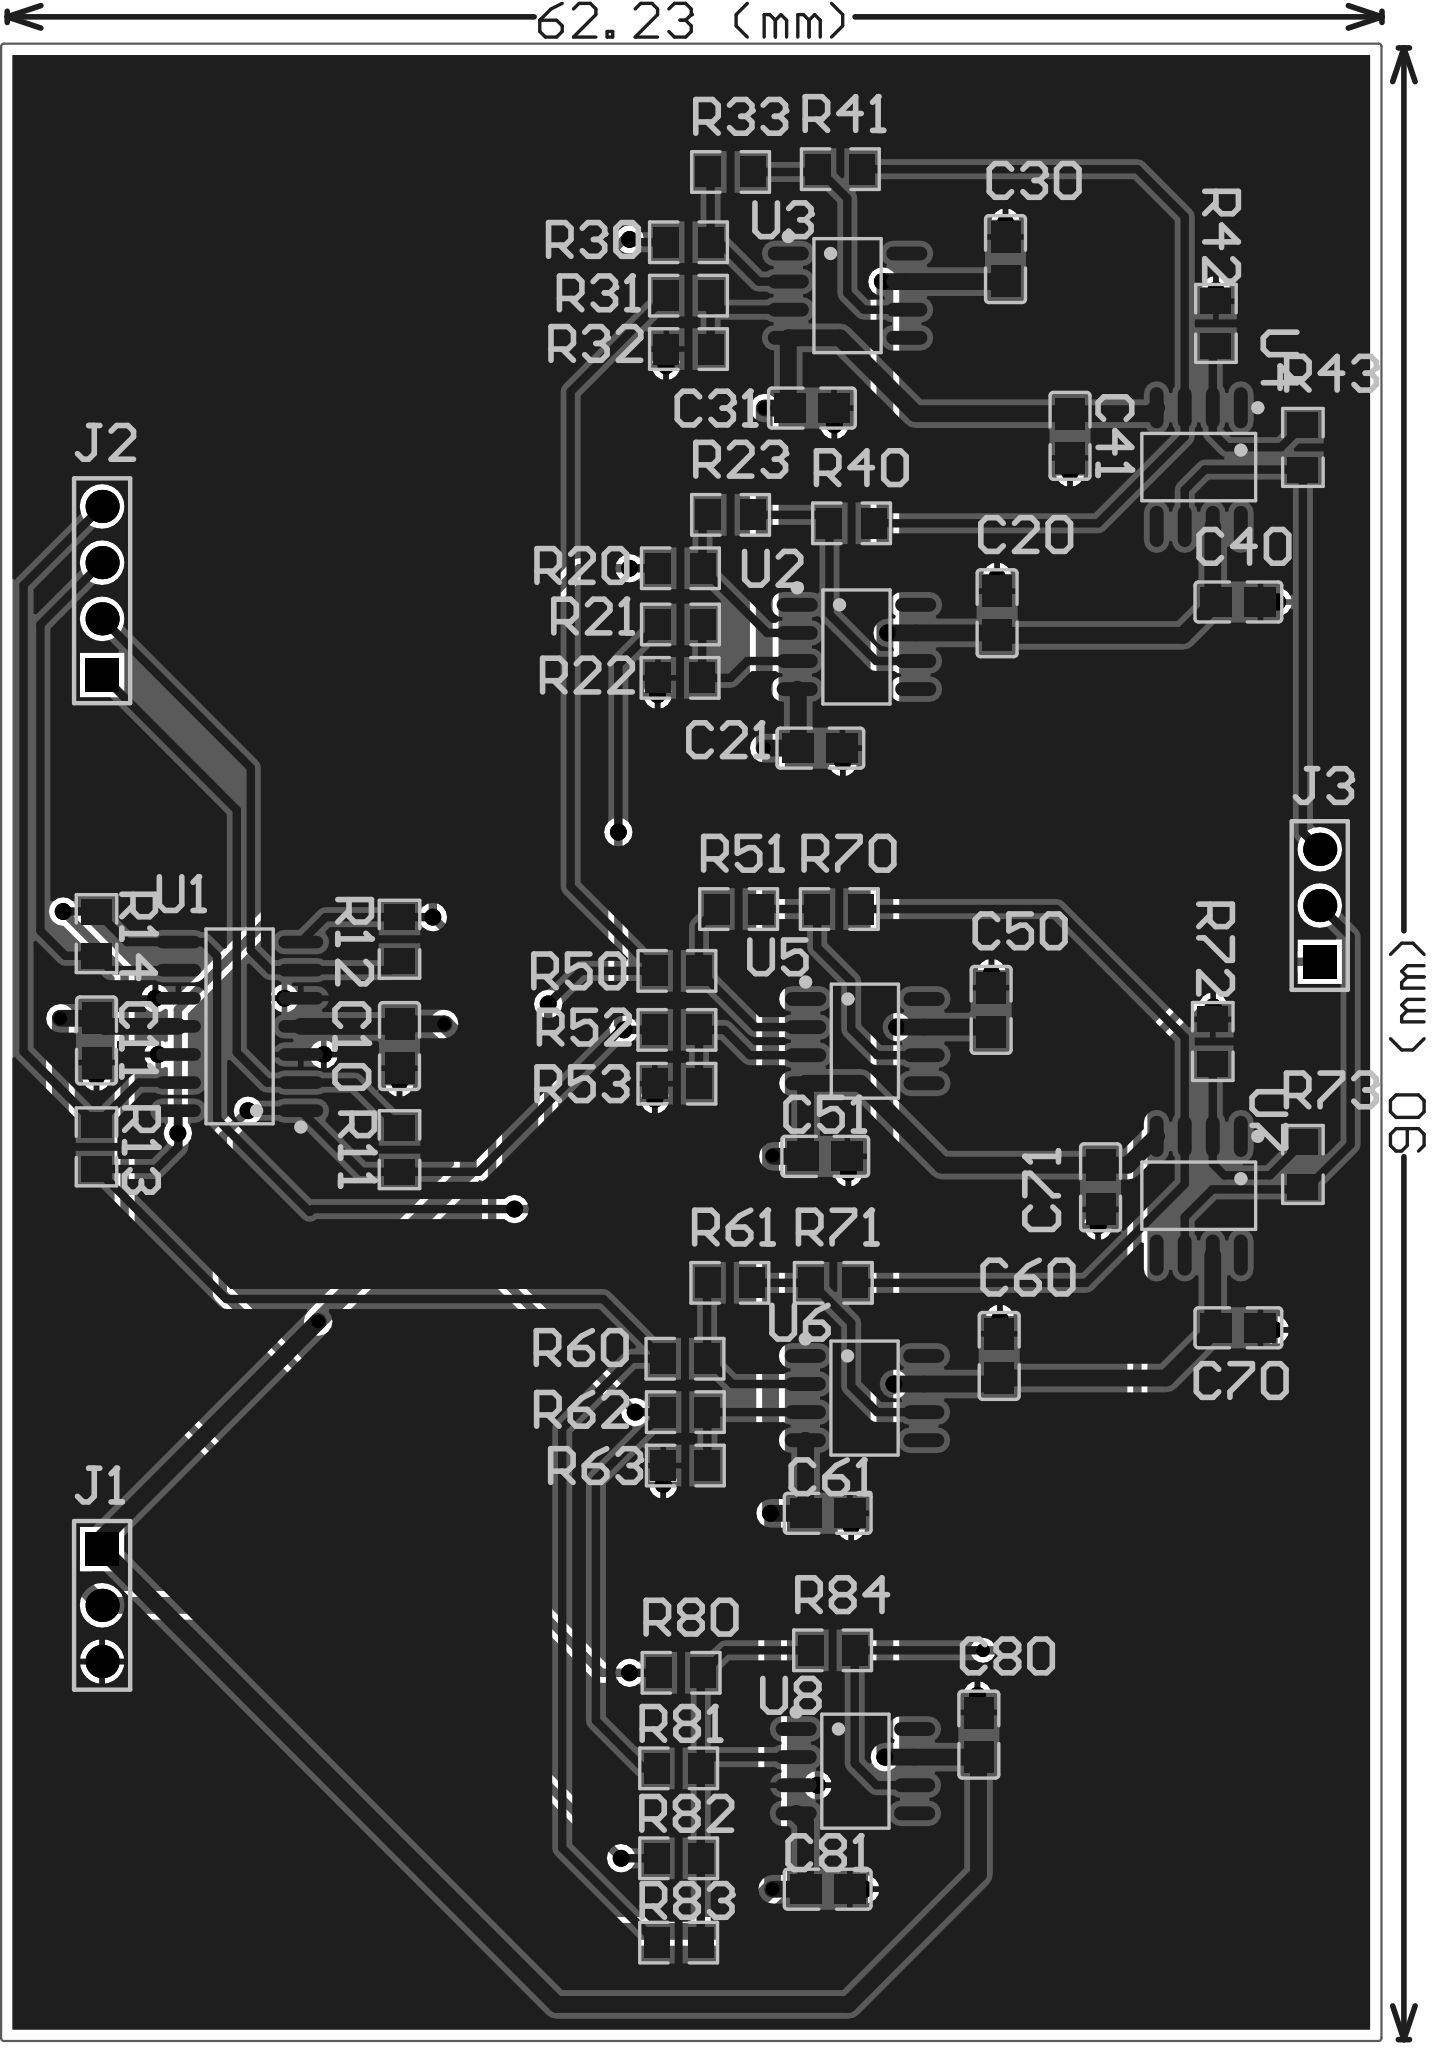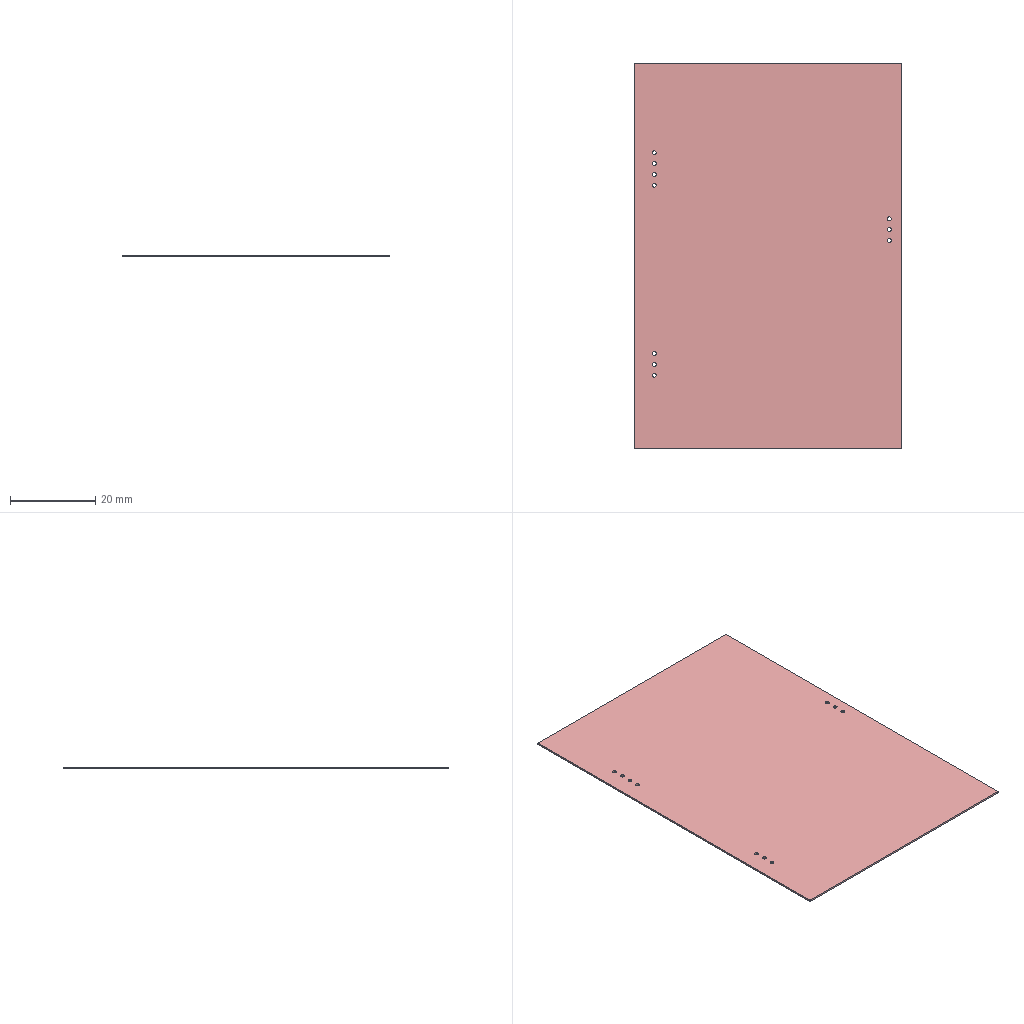Circuit board layout | Altium Designer | box 62.5 x 90.3 x 0.4 mm
Layer stack:
# Altium Designer layer stack of  (unit mm; dielectric type: 0 none, 1 core, 2 prepreg, 3 surface material)
index,name,kind,layer,copper_thickness_mm,dielectric_type,dielectric_thickness_mm,dielectric_material,dielectric_constant
0,Top Paste,other,,,,,,
1,Top Overlay,other,,,,,,
2,Top Solder,dielectric,,,3,0.0102,Solder Resist,3.5
3,Top Layer,copper,Top Layer,0.0356,,,,
4,Dielectric 1,dielectric,,,0,0.32,FR-4,4.8
5,Bottom Layer,copper,Bottom Layer,0.0356,,,,
6,Bottom Solder,dielectric,,,3,0.0102,Solder Resist,3.5
7,Bottom Overlay,other,,,,,,
8,Bottom Paste,other,,,,,,
# drill layer pairs: low layer,high layer
drill_pair,Top Layer,Bottom Layer
Part placement:
Designator,Comment,Layer,Footprint,Center-X(mm),Center-Y(mm),Rotation
U8,OP07,TopLayer,SOP-8_L4.9-W3.9-P1.27-LS6.0-BL,75.501,37.465,270
U7,OP07,TopLayer,SOP-8_L4.9-W3.9-P1.27-LS6.0-BL,91.043,63.468,180
U6,OP07,TopLayer,SOP-8_L4.9-W3.9-P1.27-LS6.0-BL,75.914,54.324,270
U5,OP07,TopLayer,SOP-8_L4.9-W3.9-P1.27-LS6.0-BL,75.93,70.453,270
U4,OP07,TopLayer,SOP-8_L4.9-W3.9-P1.27-LS6.0-BL,91.043,96.393,180
U3,OP07,TopLayer,SOP-8_L4.9-W3.9-P1.27-LS6.0-BL,75.145,104.14,270
U2,OP07,TopLayer,SOP-8_L4.9-W3.9-P1.27-LS6.0-BL,75.549,88.265,270
U1,OPA4131,TopLayer,SOIC-14_L8.7-W3.9-P1.27-LS6.0-BL,47.625,71.12,90
R84,10k,TopLayer,R0805,74.469,42.926,360
R83,10k,TopLayer,R0805,67.5,29.718,360
R82,10k,TopLayer,R0805,67.5,33.528,360
R81,10k,TopLayer,R0805,67.5,37.592,360
R80,10k,TopLayer,R0805,67.611,41.91,360
R73,10K,TopLayer,R0805,95.758,64.881,90
R72,10K,TopLayer,R0805,91.678,70.437,270
R71,10K,TopLayer,R0805,74.501,59.531,360
R70,10K,TopLayer,R0805,74.771,76.422,360
R63,10K,TopLayer,R0805,67.802,51.276,360
R62,10K,TopLayer,R0805,67.802,53.689,360
R61,10K,TopLayer,R0805,69.818,59.531,360
R60,10K,TopLayer,R0805,67.786,56.102,360
R53,10K,TopLayer,R0805,67.421,68.53,360
R52,10K,TopLayer,R0805,67.421,70.961,360
R51,10K,TopLayer,R0805,70.215,76.422,360
R50,10K,TopLayer,R0805,67.421,73.628,360
R43,10K,TopLayer,R0805,95.758,97.282,90
R42,10K,TopLayer,R0805,91.821,102.886,270
R41,10K,TopLayer,R0805,74.819,109.855,360
R40,10K,TopLayer,R0805,75.327,93.853,360
R33,10K,TopLayer,R0805,69.85,109.728,360
R32,10K,TopLayer,R0805,67.945,101.727,360
R31,10K,TopLayer,R0805,67.945,104.14,360
R30,10K,TopLayer,R0805,67.945,106.553,360
R23,10K,TopLayer,R0805,69.85,94.234,360
R22,10K,TopLayer,R0805,67.564,86.868,360
R21,10K,TopLayer,R0805,67.58,89.281,360
R20,10K,TopLayer,R0805,67.58,91.821,360
R14,3K,TopLayer,R0805,41.148,75.311,270
R13,3K,TopLayer,R0805,41.148,65.675,90
R12,3K,TopLayer,R0805,54.864,75.057,90
R11,3K,TopLayer,R0805,54.864,65.548,270
J3,输出,TopLayer,HDR1X3,96.52,76.581,90
J2,四路信号输入,TopLayer,HDR1X4,41.402,90.805,90
J1,电源,TopLayer,HDR1X3,41.402,44.958,270
C81,0.1uF,TopLayer,C0805,74.247,32.131,360
C80,0.1uF,TopLayer,C0805,81.089,39.116,90
C71,0.1uF,TopLayer,C0805,86.598,63.849,270
C70,0.1uF,TopLayer,C0805,92.837,57.499,360
C61,0.1uF,TopLayer,C0805,74.247,49.117,360
C60,0.1uF,TopLayer,C0805,82.01,56.229,90
C51,0.1uF,TopLayer,C0805,74.136,65.246,360
C50,0.1uF,TopLayer,C0805,81.645,71.866,90
C41,0.1uF,TopLayer,C0805,85.217,97.806,270
C40,0.1uF,TopLayer,C0805,92.837,90.297,360
C31,0.1uF,TopLayer,C0805,73.533,99.06,360
C30,0.1uF,TopLayer,C0805,82.296,105.791,90
C21,0.1uF,TopLayer,C0805,73.914,83.693,0
C20,0.1uF,TopLayer,C0805,81.915,89.789,90
C11,0.1uF,TopLayer,C0805,41.148,70.485,90
C10,0.1uF,TopLayer,C0805,54.864,70.231,90
Pad and via stacks:
# Altium Designer via and pad stacks of  (unit mm). Each distinct definition once, with the count of objects using it.
# via: kind,start_layer,end_layer,hole_mm,diameter_mm,mode(0 simple;1 top-mid-bottom;2 full stack),diameter_per_layer,count,example_net
# pad: kind,layer,hole_mm,hole_type(0 round;1 square;2 slot),plating,top_size,top_shape(1 round;2 rect;3 octagon;9 rounded rect),mid_size,bottom_size,mode,footprint,size_per_layer,count,example
pad,Top Layer,0,0,plated,1.133x1.377,2,1.133x1.377,1.133x1.377,0,R0805,,66,R83.1
pad,Top Layer,0,0,plated,1.41x1.35,2,1.41x1.35,1.41x1.35,0,C0805,,32,C81.1
pad,Top Layer,0,0,plated,0.63x1.865,1,0.63x1.865,0.63x1.865,0,SOP-8_L4.9-W3.9-P1.27-LS6.0-BL,,56,U8.5
pad,Top Layer,0,0,plated,0.574x2.038,1,0.574x2.038,0.574x2.038,0,SOIC-14_L8.7-W3.9-P1.27-LS6.0-BL,,14,U1.8
pad,Multi-Layer,0.9,0,plated,1.5x1.5,2,1.5x1.5,1.5x1.5,0,HDR1X3,,2,J3.1
pad,Multi-Layer,0.9,0,plated,1.5x1.5,1,1.5x1.5,1.5x1.5,0,HDR1X3,,4,J3.2
pad,Multi-Layer,0.9,0,plated,1.5x1.5,1,1.5x1.5,1.5x1.5,0,HDR1X4,,3,J2.4
pad,Multi-Layer,0.9,0,plated,1.5x1.5,2,1.5x1.5,1.5x1.5,0,HDR1X4,,1,J2.1
via,Top Layer,Bottom Layer,0.3048,0.6096,0,,8,+15V
via,Top Layer,Bottom Layer,0.381,0.762,0,,46,OutC
Copper pours:
name,layer,net,type(0 solid;1 hatched;2 none)
G,Bottom Layer,GND,0
G,Top Layer,GND,0
Design rules, without the lines most boards share:
# Altium Designer design rules of  (exported by Altium Designer, unit mm)
# columns: name | kind | enabled | priority | scope1 | scope2 | descriptor | typed fields (field=value)
NetAntennae | 56 | enabled | 1 | All | All | Net Antennae (Tolerance=0mm) (All) |
SilkToSilkClearance | 55 | enabled | 1 | All | All | Silk to Silk (Clearance=0mm) (All),(All) |
SilkToSolderMaskClearance | 54 | enabled | 1 | IsPad | All | Silk To Solder Mask (Clearance=0mm) (IsPad),(All) |
MinimumSolderMaskSliver | 53 | enabled | 1 | All | All | Minimum Solder Mask Sliver (Gap=0mm) (All),(All) |
HoleToHoleClearance | 52 | enabled | 1 | All | All | Hole To Hole Clearance (Gap=0.254mm) (All),(All) | gap=0.254
DiffPairsRouting | 51 | enabled | 1 | All | All | Differential Pairs Uncoupled Length using the Gap Constraints (Min=0.254mm) (Max=0.254mm) (Prefered=0.254mm)  and Width Constraints (Min=0.381mm) (Max=0.381mm) (Prefered=0.381mm) (All) |
HoleSize | 42 | enabled | 1 | All | All | Hole Size Constraint (Min=0.025mm) (Max=2.54mm) (All) |
Height | 50 | enabled | 1 | All | All | Height Constraint (Min=0mm) (Max=25.4mm) (Prefered=12.7mm) (All) | min_height=0 max_height=25.4
ComponentClearance | 24 | enabled | 1 | All | All | Component Clearance Constraint ( Horizontal Gap = 0.254mm, Vertical Gap = 0.254mm ) (All),(All)  | gap=0.254
SolderMaskExpansion | 13 | enabled | 1 | All | All | Solder Mask Expansion (Expansion =0.102mm) (All) | expansion=0.1016
PasteMaskExpansion | 14 | enabled | 1 | All | All | Paste Mask Expansion (Expansion =0mm) (All) | expansion=0
RoutingVias | 11 | enabled | 1 | All | All | Routing Via (MinHoleWidth=0.711mm) (MaxHoleWidth=0.711mm) (PreferredHoleWidth=0.711mm) (MinWidth=1.27mm) (MaxWidth=1.27mm) (PreferedWidth=1.27mm) (All) | via_min_hole=0.7112 via_max_hole=0.7112 via_preferred_diameter=1.27 via_preferred_hole=0.7112
RoutingCorners | 10 | enabled | 1 | All | All | Routing Corners (Style=45-Degree) (Min Setback=2.54mm) (Max Setback=2.54mm) (All) |
Width | 2 | enabled | 1 | All | All | Width Constraint (Min=0.254mm) (Max=0.762mm) (Preferred=0.254mm) (All) |
PolygonConnect | 20 | enabled | 1 | All | All | Polygon Connect Rule(Relief Connect )(Conductor Width=0.254mm) (Relief Angle=90 Angle) (Entries=4) (Air Gap Width=0.254mm) (All),(All) | connect_style(0=relief,1=direct,2=none)=0 relief_conductor_width=0.254 relief_entries=4
PlaneClearance | 12 | enabled | 1 | All | All | Power Plane Clearance (Clearance =0.508mm) (All) | clearance=0.508
PlaneConnect | 6 | enabled | 1 | All | All | Power Plane Connect Rule(Relief Connect )(Expansion=0.508mm) (Conductor Width=0.254mm) (Air Gap=0.254mm) (Entries=4) (All) | relief_conductor_width=0.254 relief_entries=4 relief_expansion=0.508
Clearance | 0 | enabled | 1 | All | All | Clearance Constraint (Gap=0.254mm) (All),(All) | gap=0.254
Classes set for this board:
# Altium Designer classes of  (member kind: 0 net, 1 component, 2 from-to, 3 pad, 4 layer, 5 differential pair, 6 design channel, 7 polygon, 8 structure, 9 xSignal)
# columns: class name | member kind | superclass | members
normalization_processing | 1 | no | C10; C11; C20; C21; C30; C31; C40; C41; C50; C51; C60; C61; C70; C71; C80; C81; J1; J2; J3; R11; R12; R13; R14; R20; R21; R22; R23; R30; R31; R32; R33; R40; R41; R42; R43; R50; R51; R52; R53; R60; R61; R62; R63; R70; R71; R72; R73; R80; R81; R82; R83; R84; U1; U2; U3; U4; U5; U6; U7; U8;